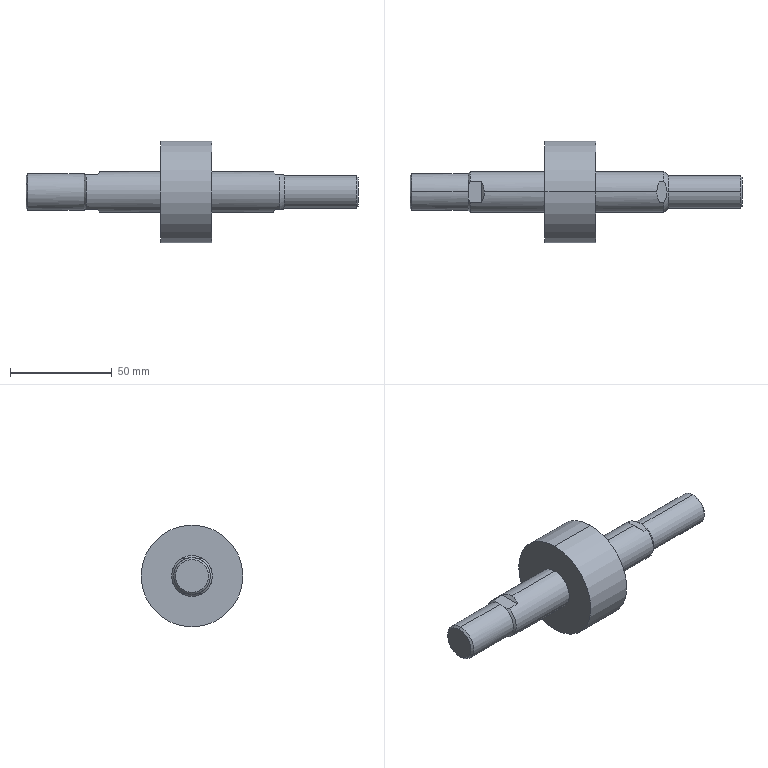Part | SolidWorks | features BaseBody 1 | 1 solid | 32 faces | box 163 x 50 x 50 mm | volume 86233 mm3 | plane 14 | cylinder 10 | cone 8 | commonest cylinder face diameters 20 x4 16 x2 18 x2 50 x2
STEP:
#1=CARTESIAN_POINT('',(57.75,0.,25.));
#2=VERTEX_POINT('',#1);
#3=CARTESIAN_POINT('',(57.75,0.,-25.));
#4=VERTEX_POINT('',#3);
#5=CARTESIAN_POINT('',(57.75,0.,0.));
#6=DIRECTION('',(-1.,0.,0.));
#7=DIRECTION('',(0.,0.,1.));
#8=AXIS2_PLACEMENT_3D('',#5,#6,#7);
#9=CIRCLE('',#8,25.);
#10=EDGE_CURVE('',#2,#4,#9,.T.);
#11=ORIENTED_EDGE('',*,*,#10,.T.);
#12=CARTESIAN_POINT('',(32.75,0.,-25.));
#13=VERTEX_POINT('',#12);
#14=CARTESIAN_POINT('',(57.75,0.,-25.));
#15=DIRECTION('',(-1.,0.,0.));
#16=VECTOR('',#15,1000.);
#17=LINE('',#14,#16);
#18=EDGE_CURVE('',#4,#13,#17,.T.);
#19=ORIENTED_EDGE('',*,*,#18,.T.);
#20=CARTESIAN_POINT('',(32.75,0.,25.));
#21=VERTEX_POINT('',#20);
#22=CARTESIAN_POINT('',(32.75,0.,0.));
#23=DIRECTION('',(1.,0.,0.));
#24=DIRECTION('',(0.,0.,1.));
#25=AXIS2_PLACEMENT_3D('',#22,#23,#24);
#26=CIRCLE('',#25,25.);
#27=EDGE_CURVE('',#13,#21,#26,.T.);
#28=ORIENTED_EDGE('',*,*,#27,.T.);
#29=CARTESIAN_POINT('',(57.75,0.,25.));
#30=DIRECTION('',(-1.,0.,0.));
#31=VECTOR('',#30,1000.);
#32=LINE('',#29,#31);
#33=EDGE_CURVE('',#2,#21,#32,.T.);
#34=ORIENTED_EDGE('',*,*,#33,.F.);
#35=EDGE_LOOP('',(#11,#19,#28,#34));
#36=FACE_OUTER_BOUND('',#35,.T.);
#37=CARTESIAN_POINT('',(57.75,0.,0.));
#38=DIRECTION('',(-1.,0.,0.));
#39=DIRECTION('',(0.,0.,1.));
#40=AXIS2_PLACEMENT_3D('',#37,#38,#39);
#41=CYLINDRICAL_SURFACE('',#40,25.);
#42=ADVANCED_FACE('',(#36),#41,.T.);
#43=CARTESIAN_POINT('',(32.75,0.,10.));
#44=VERTEX_POINT('',#43);
#45=CARTESIAN_POINT('',(32.75,0.,-10.));
#46=VERTEX_POINT('',#45);
#47=CARTESIAN_POINT('',(32.75,0.,0.));
#48=DIRECTION('',(-1.,0.,0.));
#49=DIRECTION('',(0.,0.,1.));
#50=AXIS2_PLACEMENT_3D('',#47,#48,#49);
#51=CIRCLE('',#50,10.);
#52=EDGE_CURVE('',#44,#46,#51,.T.);
#53=ORIENTED_EDGE('',*,*,#52,.T.);
#54=CARTESIAN_POINT('',(3.,0.,-10.));
#55=VERTEX_POINT('',#54);
#56=CARTESIAN_POINT('',(57.75,0.,-10.));
#57=DIRECTION('',(-1.,0.,0.));
#58=VECTOR('',#57,1000.);
#59=LINE('',#56,#58);
#60=EDGE_CURVE('',#46,#55,#59,.T.);
#61=ORIENTED_EDGE('',*,*,#60,.T.);
#62=CARTESIAN_POINT('',(1.5,5.268,-8.5));
#63=VERTEX_POINT('',#62);
#64=CARTESIAN_POINT('',(3.,0.,-10.));
#65=CARTESIAN_POINT('',(3.,1.873,-10.));
#66=CARTESIAN_POINT('',(2.487,3.675,-9.487));
#67=CARTESIAN_POINT('',(1.5,5.268,-8.5));
#68=(BOUNDED_CURVE()B_SPLINE_CURVE(3,(#64,#65,#66,#67),.UNSPECIFIED.,.F.,.F.)B_SPLINE_CURVE_WITH_KNOTS((4,4),(3.142,3.696),.UNSPECIFIED.)CURVE()GEOMETRIC_REPRESENTATION_ITEM()RATIONAL_B_SPLINE_CURVE((1.,0.9745,0.9745,1.))REPRESENTATION_ITEM(''));
#69=EDGE_CURVE('',#55,#63,#68,.T.);
#70=ORIENTED_EDGE('',*,*,#69,.T.);
#71=CARTESIAN_POINT('',(-4.,5.268,-8.5));
#72=VERTEX_POINT('',#71);
#73=CARTESIAN_POINT('',(57.75,5.268,-8.5));
#74=DIRECTION('',(-1.,0.,0.));
#75=VECTOR('',#74,1000.);
#76=LINE('',#73,#75);
#77=EDGE_CURVE('',#63,#72,#76,.T.);
#78=ORIENTED_EDGE('',*,*,#77,.T.);
#79=CARTESIAN_POINT('',(-4.,5.268,8.5));
#80=VERTEX_POINT('',#79);
#81=CARTESIAN_POINT('',(-4.,0.,0.));
#82=DIRECTION('',(1.,0.,0.));
#83=DIRECTION('',(0.,0.,1.));
#84=AXIS2_PLACEMENT_3D('',#81,#82,#83);
#85=CIRCLE('',#84,10.);
#86=EDGE_CURVE('',#72,#80,#85,.T.);
#87=ORIENTED_EDGE('',*,*,#86,.T.);
#88=CARTESIAN_POINT('',(1.5,5.268,8.5));
#89=VERTEX_POINT('',#88);
#90=CARTESIAN_POINT('',(57.75,5.268,8.5));
#91=DIRECTION('',(1.,0.,0.));
#92=VECTOR('',#91,1000.);
#93=LINE('',#90,#92);
#94=EDGE_CURVE('',#80,#89,#93,.T.);
#95=ORIENTED_EDGE('',*,*,#94,.T.);
#96=CARTESIAN_POINT('',(3.,0.,10.));
#97=VERTEX_POINT('',#96);
#98=CARTESIAN_POINT('',(1.5,5.268,8.5));
#99=CARTESIAN_POINT('',(2.487,3.675,9.487));
#100=CARTESIAN_POINT('',(3.,1.873,10.));
#101=CARTESIAN_POINT('',(3.,0.,10.));
#102=(BOUNDED_CURVE()B_SPLINE_CURVE(3,(#98,#99,#100,#101),.UNSPECIFIED.,.F.,.F.)B_SPLINE_CURVE_WITH_KNOTS((4,4),(2.587,3.142),.UNSPECIFIED.)CURVE()GEOMETRIC_REPRESENTATION_ITEM()RATIONAL_B_SPLINE_CURVE((1.,0.9745,0.9745,1.))REPRESENTATION_ITEM(''));
#103=EDGE_CURVE('',#89,#97,#102,.T.);
#104=ORIENTED_EDGE('',*,*,#103,.T.);
#105=CARTESIAN_POINT('',(57.75,0.,10.));
#106=DIRECTION('',(-1.,0.,0.));
#107=VECTOR('',#106,1000.);
#108=LINE('',#105,#107);
#109=EDGE_CURVE('',#44,#97,#108,.T.);
#110=ORIENTED_EDGE('',*,*,#109,.F.);
#111=EDGE_LOOP('',(#53,#61,#70,#78,#87,#95,#104,#110));
#112=FACE_OUTER_BOUND('',#111,.T.);
#113=CARTESIAN_POINT('',(57.75,0.,0.));
#114=DIRECTION('',(-1.,0.,0.));
#115=DIRECTION('',(0.,0.,1.));
#116=AXIS2_PLACEMENT_3D('',#113,#114,#115);
#117=CYLINDRICAL_SURFACE('',#116,10.);
#118=ADVANCED_FACE('',(#112),#117,.T.);
#119=CARTESIAN_POINT('',(89.2,5.268,-8.5));
#120=VERTEX_POINT('',#119);
#121=CARTESIAN_POINT('',(87.7,0.,-10.));
#122=VERTEX_POINT('',#121);
#123=CARTESIAN_POINT('',(89.2,5.268,-8.5));
#124=CARTESIAN_POINT('',(88.213,3.675,-9.487));
#125=CARTESIAN_POINT('',(87.7,1.873,-10.));
#126=CARTESIAN_POINT('',(87.7,0.,-10.));
#127=(BOUNDED_CURVE()B_SPLINE_CURVE(3,(#123,#124,#125,#126),.UNSPECIFIED.,.F.,.F.)B_SPLINE_CURVE_WITH_KNOTS((4,4),(5.728,6.283),.UNSPECIFIED.)CURVE()GEOMETRIC_REPRESENTATION_ITEM()RATIONAL_B_SPLINE_CURVE((1.,0.9745,0.9745,1.))REPRESENTATION_ITEM(''));
#128=EDGE_CURVE('',#120,#122,#127,.T.);
#129=ORIENTED_EDGE('',*,*,#128,.T.);
#130=CARTESIAN_POINT('',(57.75,0.,-10.));
#131=VERTEX_POINT('',#130);
#132=CARTESIAN_POINT('',(129.5,0.,-10.));
#133=DIRECTION('',(-1.,0.,0.));
#134=VECTOR('',#133,1000.);
#135=LINE('',#132,#134);
#136=EDGE_CURVE('',#122,#131,#135,.T.);
#137=ORIENTED_EDGE('',*,*,#136,.T.);
#138=CARTESIAN_POINT('',(57.75,0.,10.));
#139=VERTEX_POINT('',#138);
#140=CARTESIAN_POINT('',(57.75,0.,0.));
#141=DIRECTION('',(1.,0.,0.));
#142=DIRECTION('',(0.,0.,1.));
#143=AXIS2_PLACEMENT_3D('',#140,#141,#142);
#144=CIRCLE('',#143,10.);
#145=EDGE_CURVE('',#131,#139,#144,.T.);
#146=ORIENTED_EDGE('',*,*,#145,.T.);
#147=CARTESIAN_POINT('',(87.7,0.,10.));
#148=VERTEX_POINT('',#147);
#149=CARTESIAN_POINT('',(129.5,0.,10.));
#150=DIRECTION('',(-1.,0.,0.));
#151=VECTOR('',#150,1000.);
#152=LINE('',#149,#151);
#153=EDGE_CURVE('',#148,#139,#152,.T.);
#154=ORIENTED_EDGE('',*,*,#153,.F.);
#155=CARTESIAN_POINT('',(89.2,5.268,8.5));
#156=VERTEX_POINT('',#155);
#157=CARTESIAN_POINT('',(87.7,0.,10.));
#158=CARTESIAN_POINT('',(87.7,1.873,10.));
#159=CARTESIAN_POINT('',(88.213,3.675,9.487));
#160=CARTESIAN_POINT('',(89.2,5.268,8.5));
#161=(BOUNDED_CURVE()B_SPLINE_CURVE(3,(#157,#158,#159,#160),.UNSPECIFIED.,.F.,.F.)B_SPLINE_CURVE_WITH_KNOTS((4,4),(0.,0.5548),.UNSPECIFIED.)CURVE()GEOMETRIC_REPRESENTATION_ITEM()RATIONAL_B_SPLINE_CURVE((1.,0.9745,0.9745,1.))REPRESENTATION_ITEM(''));
#162=EDGE_CURVE('',#148,#156,#161,.T.);
#163=ORIENTED_EDGE('',*,*,#162,.T.);
#164=CARTESIAN_POINT('',(91.2,5.268,8.5));
#165=VERTEX_POINT('',#164);
#166=CARTESIAN_POINT('',(129.5,5.268,8.5));
#167=DIRECTION('',(1.,0.,0.));
#168=VECTOR('',#167,1000.);
#169=LINE('',#166,#168);
#170=EDGE_CURVE('',#156,#165,#169,.T.);
#171=ORIENTED_EDGE('',*,*,#170,.T.);
#172=CARTESIAN_POINT('',(91.2,5.268,-8.5));
#173=VERTEX_POINT('',#172);
#174=CARTESIAN_POINT('',(91.2,0.,0.));
#175=DIRECTION('',(-1.,0.,0.));
#176=DIRECTION('',(0.,0.,1.));
#177=AXIS2_PLACEMENT_3D('',#174,#175,#176);
#178=CIRCLE('',#177,10.);
#179=EDGE_CURVE('',#165,#173,#178,.T.);
#180=ORIENTED_EDGE('',*,*,#179,.T.);
#181=CARTESIAN_POINT('',(129.5,5.268,-8.5));
#182=DIRECTION('',(-1.,0.,0.));
#183=VECTOR('',#182,1000.);
#184=LINE('',#181,#183);
#185=EDGE_CURVE('',#173,#120,#184,.T.);
#186=ORIENTED_EDGE('',*,*,#185,.T.);
#187=EDGE_LOOP('',(#129,#137,#146,#154,#163,#171,#180,#186));
#188=FACE_OUTER_BOUND('',#187,.T.);
#189=CARTESIAN_POINT('',(129.5,0.,0.));
#190=DIRECTION('',(-1.,0.,0.));
#191=DIRECTION('',(0.,0.,1.));
#192=AXIS2_PLACEMENT_3D('',#189,#190,#191);
#193=CYLINDRICAL_SURFACE('',#192,10.);
#194=ADVANCED_FACE('',(#188),#193,.T.);
#195=CARTESIAN_POINT('',(93.2,0.,8.));
#196=VERTEX_POINT('',#195);
#197=CARTESIAN_POINT('',(93.2,0.,-8.));
#198=VERTEX_POINT('',#197);
#199=CARTESIAN_POINT('',(93.2,0.,0.));
#200=DIRECTION('',(-1.,0.,0.));
#201=DIRECTION('',(0.,0.,1.));
#202=AXIS2_PLACEMENT_3D('',#199,#200,#201);
#203=CIRCLE('',#202,8.);
#204=EDGE_CURVE('',#196,#198,#203,.T.);
#205=ORIENTED_EDGE('',*,*,#204,.T.);
#206=CARTESIAN_POINT('',(92.7,0.,-8.5));
#207=VERTEX_POINT('',#206);
#208=CARTESIAN_POINT('',(91.2,0.,-10.));
#209=DIRECTION('',(-0.7071,0.,-0.7071));
#210=VECTOR('',#209,1000.);
#211=LINE('',#208,#210);
#212=EDGE_CURVE('',#198,#207,#211,.T.);
#213=ORIENTED_EDGE('',*,*,#212,.T.);
#214=CARTESIAN_POINT('',(92.7,0.,-8.5));
#215=CARTESIAN_POINT('',(92.7,0.459,-8.5));
#216=CARTESIAN_POINT('',(92.663,0.9179,-8.5));
#217=CARTESIAN_POINT('',(92.516,1.835,-8.5));
#218=CARTESIAN_POINT('',(92.408,2.287,-8.5));
#219=CARTESIAN_POINT('',(92.005,3.607,-8.5));
#220=CARTESIAN_POINT('',(91.632,4.448,-8.5));
#221=CARTESIAN_POINT('',(91.2,5.268,-8.5));
#222=B_SPLINE_CURVE_WITH_KNOTS('',3,(#214,#215,#216,#217,#218,#219,#220,#221),.UNSPECIFIED.,.F.,.F.,(4,2,2,4),(0.005508,0.006884,0.008261,0.01101),.UNSPECIFIED.);
#223=EDGE_CURVE('',#207,#173,#222,.T.);
#224=ORIENTED_EDGE('',*,*,#223,.T.);
#225=ORIENTED_EDGE('',*,*,#179,.F.);
#226=CARTESIAN_POINT('',(92.7,0.,8.5));
#227=VERTEX_POINT('',#226);
#228=CARTESIAN_POINT('',(92.7,0.,8.5));
#229=CARTESIAN_POINT('',(92.7,0.459,8.5));
#230=CARTESIAN_POINT('',(92.663,0.9179,8.5));
#231=CARTESIAN_POINT('',(92.516,1.835,8.5));
#232=CARTESIAN_POINT('',(92.408,2.287,8.5));
#233=CARTESIAN_POINT('',(92.005,3.607,8.5));
#234=CARTESIAN_POINT('',(91.632,4.448,8.5));
#235=CARTESIAN_POINT('',(91.2,5.268,8.5));
#236=B_SPLINE_CURVE_WITH_KNOTS('',3,(#228,#229,#230,#231,#232,#233,#234,#235),.UNSPECIFIED.,.F.,.F.,(4,2,2,4),(0.005508,0.006884,0.008261,0.01101),.UNSPECIFIED.);
#237=EDGE_CURVE('',#227,#165,#236,.T.);
#238=ORIENTED_EDGE('',*,*,#237,.F.);
#239=CARTESIAN_POINT('',(91.2,0.,10.));
#240=DIRECTION('',(-0.7071,0.,0.7071));
#241=VECTOR('',#240,1000.);
#242=LINE('',#239,#241);
#243=EDGE_CURVE('',#196,#227,#242,.T.);
#244=ORIENTED_EDGE('',*,*,#243,.F.);
#245=EDGE_LOOP('',(#205,#213,#224,#225,#238,#244));
#246=FACE_OUTER_BOUND('',#245,.T.);
#247=CARTESIAN_POINT('',(91.2,0.,0.));
#248=DIRECTION('',(-1.,0.,0.));
#249=DIRECTION('',(0.,0.,1.));
#250=AXIS2_PLACEMENT_3D('',#247,#248,#249);
#251=CONICAL_SURFACE('',#250,10.,0.7854);
#252=ADVANCED_FACE('',(#246),#251,.T.);
#253=CARTESIAN_POINT('',(-5.,2.958,-8.5));
#254=VERTEX_POINT('',#253);
#255=CARTESIAN_POINT('',(-5.,0.,-9.));
#256=VERTEX_POINT('',#255);
#257=CARTESIAN_POINT('',(-5.,0.,0.));
#258=DIRECTION('',(-1.,0.,0.));
#259=DIRECTION('',(0.,0.,1.));
#260=AXIS2_PLACEMENT_3D('',#257,#258,#259);
#261=CIRCLE('',#260,9.);
#262=EDGE_CURVE('',#254,#256,#261,.T.);
#263=ORIENTED_EDGE('',*,*,#262,.T.);
#264=CARTESIAN_POINT('',(-32.58,0.,-9.));
#265=VERTEX_POINT('',#264);
#266=CARTESIAN_POINT('',(0.,0.,-9.));
#267=DIRECTION('',(-1.,0.,0.));
#268=VECTOR('',#267,1000.);
#269=LINE('',#266,#268);
#270=EDGE_CURVE('',#256,#265,#269,.T.);
#271=ORIENTED_EDGE('',*,*,#270,.T.);
#272=CARTESIAN_POINT('',(-32.58,0.,9.));
#273=VERTEX_POINT('',#272);
#274=CARTESIAN_POINT('',(-32.58,0.,0.));
#275=DIRECTION('',(1.,0.,0.));
#276=DIRECTION('',(0.,0.,1.));
#277=AXIS2_PLACEMENT_3D('',#274,#275,#276);
#278=CIRCLE('',#277,9.);
#279=EDGE_CURVE('',#265,#273,#278,.T.);
#280=ORIENTED_EDGE('',*,*,#279,.T.);
#281=CARTESIAN_POINT('',(-5.,0.,9.));
#282=VERTEX_POINT('',#281);
#283=CARTESIAN_POINT('',(0.,0.,9.));
#284=DIRECTION('',(-1.,0.,0.));
#285=VECTOR('',#284,1000.);
#286=LINE('',#283,#285);
#287=EDGE_CURVE('',#282,#273,#286,.T.);
#288=ORIENTED_EDGE('',*,*,#287,.F.);
#289=CARTESIAN_POINT('',(-5.,2.958,8.5));
#290=VERTEX_POINT('',#289);
#291=CARTESIAN_POINT('',(-5.,0.,0.));
#292=DIRECTION('',(1.,0.,0.));
#293=DIRECTION('',(0.,0.,1.));
#294=AXIS2_PLACEMENT_3D('',#291,#292,#293);
#295=CIRCLE('',#294,9.);
#296=EDGE_CURVE('',#290,#282,#295,.T.);
#297=ORIENTED_EDGE('',*,*,#296,.F.);
#298=CARTESIAN_POINT('',(-5.,0.,0.));
#299=DIRECTION('',(1.,0.,0.));
#300=DIRECTION('',(0.,0.,-1.));
#301=AXIS2_PLACEMENT_3D('',#298,#299,#300);
#302=CIRCLE('',#301,9.);
#303=EDGE_CURVE('',#254,#290,#302,.T.);
#304=ORIENTED_EDGE('',*,*,#303,.F.);
#305=EDGE_LOOP('',(#263,#271,#280,#288,#297,#304));
#306=FACE_OUTER_BOUND('',#305,.T.);
#307=CARTESIAN_POINT('',(0.,0.,0.));
#308=DIRECTION('',(-1.,0.,0.));
#309=DIRECTION('',(0.,0.,1.));
#310=AXIS2_PLACEMENT_3D('',#307,#308,#309);
#311=CYLINDRICAL_SURFACE('',#310,9.);
#312=ADVANCED_FACE('',(#306),#311,.T.);
#313=CARTESIAN_POINT('',(128.58,0.,8.));
#314=VERTEX_POINT('',#313);
#315=CARTESIAN_POINT('',(128.58,0.,-8.));
#316=VERTEX_POINT('',#315);
#317=CARTESIAN_POINT('',(128.58,0.,0.));
#318=DIRECTION('',(-1.,0.,0.));
#319=DIRECTION('',(0.,0.,1.));
#320=AXIS2_PLACEMENT_3D('',#317,#318,#319);
#321=CIRCLE('',#320,8.);
#322=EDGE_CURVE('',#314,#316,#321,.T.);
#323=ORIENTED_EDGE('',*,*,#322,.T.);
#324=CARTESIAN_POINT('',(129.5,0.,-8.));
#325=DIRECTION('',(-1.,0.,0.));
#326=VECTOR('',#325,1000.);
#327=LINE('',#324,#326);
#328=EDGE_CURVE('',#316,#198,#327,.T.);
#329=ORIENTED_EDGE('',*,*,#328,.T.);
#330=ORIENTED_EDGE('',*,*,#204,.F.);
#331=CARTESIAN_POINT('',(129.5,0.,8.));
#332=DIRECTION('',(-1.,0.,0.));
#333=VECTOR('',#332,1000.);
#334=LINE('',#331,#333);
#335=EDGE_CURVE('',#314,#196,#334,.T.);
#336=ORIENTED_EDGE('',*,*,#335,.F.);
#337=EDGE_LOOP('',(#323,#329,#330,#336));
#338=FACE_OUTER_BOUND('',#337,.T.);
#339=CARTESIAN_POINT('',(129.5,0.,0.));
#340=DIRECTION('',(-1.,0.,0.));
#341=DIRECTION('',(0.,0.,1.));
#342=AXIS2_PLACEMENT_3D('',#339,#340,#341);
#343=CYLINDRICAL_SURFACE('',#342,8.);
#344=ADVANCED_FACE('',(#338),#343,.T.);
#345=CARTESIAN_POINT('',(-33.5,0.,-8.08));
#346=VERTEX_POINT('',#345);
#347=CARTESIAN_POINT('',(-33.5,0.,8.08));
#348=VERTEX_POINT('',#347);
#349=CARTESIAN_POINT('',(-33.5,0.,0.));
#350=DIRECTION('',(1.,0.,0.));
#351=DIRECTION('',(0.,0.,-1.));
#352=AXIS2_PLACEMENT_3D('',#349,#350,#351);
#353=CIRCLE('',#352,8.08);
#354=EDGE_CURVE('',#346,#348,#353,.T.);
#355=ORIENTED_EDGE('',*,*,#354,.T.);
#356=CARTESIAN_POINT('',(-32.58,0.,9.));
#357=DIRECTION('',(0.7071,0.,0.7071));
#358=VECTOR('',#357,1000.);
#359=LINE('',#356,#358);
#360=EDGE_CURVE('',#348,#273,#359,.T.);
#361=ORIENTED_EDGE('',*,*,#360,.T.);
#362=ORIENTED_EDGE('',*,*,#279,.F.);
#363=CARTESIAN_POINT('',(-32.58,0.,-9.));
#364=DIRECTION('',(0.7071,0.,-0.7071));
#365=VECTOR('',#364,1000.);
#366=LINE('',#363,#365);
#367=EDGE_CURVE('',#346,#265,#366,.T.);
#368=ORIENTED_EDGE('',*,*,#367,.F.);
#369=EDGE_LOOP('',(#355,#361,#362,#368));
#370=FACE_OUTER_BOUND('',#369,.T.);
#371=CARTESIAN_POINT('',(-32.58,0.,0.));
#372=DIRECTION('',(1.,0.,0.));
#373=DIRECTION('',(0.,0.,-1.));
#374=AXIS2_PLACEMENT_3D('',#371,#372,#373);
#375=CONICAL_SURFACE('',#374,9.,0.7854);
#376=ADVANCED_FACE('',(#370),#375,.T.);
#377=CARTESIAN_POINT('',(129.5,0.,7.08));
#378=VERTEX_POINT('',#377);
#379=CARTESIAN_POINT('',(129.5,0.,-7.08));
#380=VERTEX_POINT('',#379);
#381=CARTESIAN_POINT('',(129.5,0.,0.));
#382=DIRECTION('',(-1.,0.,0.));
#383=DIRECTION('',(0.,0.,1.));
#384=AXIS2_PLACEMENT_3D('',#381,#382,#383);
#385=CIRCLE('',#384,7.08);
#386=EDGE_CURVE('',#378,#380,#385,.T.);
#387=ORIENTED_EDGE('',*,*,#386,.T.);
#388=CARTESIAN_POINT('',(128.58,0.,-8.));
#389=DIRECTION('',(-0.7071,0.,-0.7071));
#390=VECTOR('',#389,1000.);
#391=LINE('',#388,#390);
#392=EDGE_CURVE('',#380,#316,#391,.T.);
#393=ORIENTED_EDGE('',*,*,#392,.T.);
#394=ORIENTED_EDGE('',*,*,#322,.F.);
#395=CARTESIAN_POINT('',(128.58,0.,8.));
#396=DIRECTION('',(-0.7071,0.,0.7071));
#397=VECTOR('',#396,1000.);
#398=LINE('',#395,#397);
#399=EDGE_CURVE('',#378,#314,#398,.T.);
#400=ORIENTED_EDGE('',*,*,#399,.F.);
#401=EDGE_LOOP('',(#387,#393,#394,#400));
#402=FACE_OUTER_BOUND('',#401,.T.);
#403=CARTESIAN_POINT('',(128.58,0.,0.));
#404=DIRECTION('',(-1.,0.,0.));
#405=DIRECTION('',(0.,0.,1.));
#406=AXIS2_PLACEMENT_3D('',#403,#404,#405);
#407=CONICAL_SURFACE('',#406,8.,0.7854);
#408=ADVANCED_FACE('',(#402),#407,.T.);
#409=ORIENTED_EDGE('',*,*,#18,.F.);
#410=CARTESIAN_POINT('',(57.75,0.,0.));
#411=DIRECTION('',(-1.,0.,0.));
#412=DIRECTION('',(0.,0.,1.));
#413=AXIS2_PLACEMENT_3D('',#410,#411,#412);
#414=CIRCLE('',#413,25.);
#415=EDGE_CURVE('',#4,#2,#414,.T.);
#416=ORIENTED_EDGE('',*,*,#415,.T.);
#417=ORIENTED_EDGE('',*,*,#33,.T.);
#418=CARTESIAN_POINT('',(32.75,0.,0.));
#419=DIRECTION('',(1.,0.,0.));
#420=DIRECTION('',(0.,0.,1.));
#421=AXIS2_PLACEMENT_3D('',#418,#419,#420);
#422=CIRCLE('',#421,25.);
#423=EDGE_CURVE('',#21,#13,#422,.T.);
#424=ORIENTED_EDGE('',*,*,#423,.T.);
#425=EDGE_LOOP('',(#409,#416,#417,#424));
#426=FACE_OUTER_BOUND('',#425,.T.);
#427=CARTESIAN_POINT('',(57.75,0.,0.));
#428=DIRECTION('',(-1.,0.,0.));
#429=DIRECTION('',(0.,0.,1.));
#430=AXIS2_PLACEMENT_3D('',#427,#428,#429);
#431=CYLINDRICAL_SURFACE('',#430,25.);
#432=ADVANCED_FACE('',(#426),#431,.T.);
#433=ORIENTED_EDGE('',*,*,#52,.F.);
#434=CARTESIAN_POINT('',(32.75,0.,0.));
#435=DIRECTION('',(-1.,0.,0.));
#436=DIRECTION('',(0.,0.,1.));
#437=AXIS2_PLACEMENT_3D('',#434,#435,#436);
#438=CIRCLE('',#437,10.);
#439=EDGE_CURVE('',#46,#44,#438,.T.);
#440=ORIENTED_EDGE('',*,*,#439,.F.);
#441=EDGE_LOOP('',(#433,#440));
#442=FACE_BOUND('',#441,.T.);
#443=ORIENTED_EDGE('',*,*,#423,.F.);
#444=ORIENTED_EDGE('',*,*,#27,.F.);
#445=EDGE_LOOP('',(#443,#444));
#446=FACE_OUTER_BOUND('',#445,.T.);
#447=CARTESIAN_POINT('',(32.75,10.,0.));
#448=DIRECTION('',(1.,0.,0.));
#449=DIRECTION('',(0.,0.,-1.));
#450=AXIS2_PLACEMENT_3D('',#447,#448,#449);
#451=PLANE('',#450);
#452=ADVANCED_FACE('',(#442,#446),#451,.F.);
#453=ORIENTED_EDGE('',*,*,#10,.F.);
#454=ORIENTED_EDGE('',*,*,#415,.F.);
#455=EDGE_LOOP('',(#453,#454));
#456=FACE_OUTER_BOUND('',#455,.T.);
#457=CARTESIAN_POINT('',(57.75,0.,0.));
#458=DIRECTION('',(1.,0.,0.));
#459=DIRECTION('',(0.,0.,1.));
#460=AXIS2_PLACEMENT_3D('',#457,#458,#459);
#461=CIRCLE('',#460,10.);
#462=EDGE_CURVE('',#139,#131,#461,.T.);
#463=ORIENTED_EDGE('',*,*,#462,.F.);
#464=ORIENTED_EDGE('',*,*,#145,.F.);
#465=EDGE_LOOP('',(#463,#464));
#466=FACE_BOUND('',#465,.T.);
#467=CARTESIAN_POINT('',(57.75,25.,0.));
#468=DIRECTION('',(-1.,0.,0.));
#469=DIRECTION('',(0.,0.,1.));
#470=AXIS2_PLACEMENT_3D('',#467,#468,#469);
#471=PLANE('',#470);
#472=ADVANCED_FACE('',(#456,#466),#471,.F.);
#473=ORIENTED_EDGE('',*,*,#60,.F.);
#474=ORIENTED_EDGE('',*,*,#439,.T.);
#475=ORIENTED_EDGE('',*,*,#109,.T.);
#476=CARTESIAN_POINT('',(1.5,-5.268,8.5));
#477=VERTEX_POINT('',#476);
#478=CARTESIAN_POINT('',(3.,0.,10.));
#479=CARTESIAN_POINT('',(3.,-1.873,10.));
#480=CARTESIAN_POINT('',(2.487,-3.675,9.487));
#481=CARTESIAN_POINT('',(1.5,-5.268,8.5));
#482=(BOUNDED_CURVE()B_SPLINE_CURVE(3,(#478,#479,#480,#481),.UNSPECIFIED.,.F.,.F.)B_SPLINE_CURVE_WITH_KNOTS((4,4),(3.142,3.696),.UNSPECIFIED.)CURVE()GEOMETRIC_REPRESENTATION_ITEM()RATIONAL_B_SPLINE_CURVE((1.,0.9745,0.9745,1.))REPRESENTATION_ITEM(''));
#483=EDGE_CURVE('',#97,#477,#482,.T.);
#484=ORIENTED_EDGE('',*,*,#483,.T.);
#485=CARTESIAN_POINT('',(-4.,-5.268,8.5));
#486=VERTEX_POINT('',#485);
#487=CARTESIAN_POINT('',(57.75,-5.268,8.5));
#488=DIRECTION('',(-1.,0.,0.));
#489=VECTOR('',#488,1000.);
#490=LINE('',#487,#489);
#491=EDGE_CURVE('',#477,#486,#490,.T.);
#492=ORIENTED_EDGE('',*,*,#491,.T.);
#493=CARTESIAN_POINT('',(-4.,-5.268,-8.5));
#494=VERTEX_POINT('',#493);
#495=CARTESIAN_POINT('',(-4.,0.,0.));
#496=DIRECTION('',(1.,0.,0.));
#497=DIRECTION('',(0.,0.,1.));
#498=AXIS2_PLACEMENT_3D('',#495,#496,#497);
#499=CIRCLE('',#498,10.);
#500=EDGE_CURVE('',#486,#494,#499,.T.);
#501=ORIENTED_EDGE('',*,*,#500,.T.);
#502=CARTESIAN_POINT('',(1.5,-5.268,-8.5));
#503=VERTEX_POINT('',#502);
#504=CARTESIAN_POINT('',(57.75,-5.268,-8.5));
#505=DIRECTION('',(1.,0.,0.));
#506=VECTOR('',#505,1000.);
#507=LINE('',#504,#506);
#508=EDGE_CURVE('',#494,#503,#507,.T.);
#509=ORIENTED_EDGE('',*,*,#508,.T.);
#510=CARTESIAN_POINT('',(1.5,-5.268,-8.5));
#511=CARTESIAN_POINT('',(2.487,-3.675,-9.487));
#512=CARTESIAN_POINT('',(3.,-1.873,-10.));
#513=CARTESIAN_POINT('',(3.,0.,-10.));
#514=(BOUNDED_CURVE()B_SPLINE_CURVE(3,(#510,#511,#512,#513),.UNSPECIFIED.,.F.,.F.)B_SPLINE_CURVE_WITH_KNOTS((4,4),(2.587,3.142),.UNSPECIFIED.)CURVE()GEOMETRIC_REPRESENTATION_ITEM()RATIONAL_B_SPLINE_CURVE((1.,0.9745,0.9745,1.))REPRESENTATION_ITEM(''));
#515=EDGE_CURVE('',#503,#55,#514,.T.);
#516=ORIENTED_EDGE('',*,*,#515,.T.);
#517=EDGE_LOOP('',(#473,#474,#475,#484,#492,#501,#509,#516));
#518=FACE_OUTER_BOUND('',#517,.T.);
#519=CARTESIAN_POINT('',(57.75,0.,0.));
#520=DIRECTION('',(-1.,0.,0.));
#521=DIRECTION('',(0.,0.,1.));
#522=AXIS2_PLACEMENT_3D('',#519,#520,#521);
#523=CYLINDRICAL_SURFACE('',#522,10.);
#524=ADVANCED_FACE('',(#518),#523,.T.);
#525=ORIENTED_EDGE('',*,*,#136,.F.);
#526=CARTESIAN_POINT('',(89.2,-5.268,-8.5));
#527=VERTEX_POINT('',#526);
#528=CARTESIAN_POINT('',(87.7,0.,-10.));
#529=CARTESIAN_POINT('',(87.7,-1.873,-10.));
#530=CARTESIAN_POINT('',(88.213,-3.675,-9.487));
#531=CARTESIAN_POINT('',(89.2,-5.268,-8.5));
#532=(BOUNDED_CURVE()B_SPLINE_CURVE(3,(#528,#529,#530,#531),.UNSPECIFIED.,.F.,.F.)B_SPLINE_CURVE_WITH_KNOTS((4,4),(0.,0.5548),.UNSPECIFIED.)CURVE()GEOMETRIC_REPRESENTATION_ITEM()RATIONAL_B_SPLINE_CURVE((1.,0.9745,0.9745,1.))REPRESENTATION_ITEM(''));
#533=EDGE_CURVE('',#122,#527,#532,.T.);
#534=ORIENTED_EDGE('',*,*,#533,.T.);
#535=CARTESIAN_POINT('',(91.2,-5.268,-8.5));
#536=VERTEX_POINT('',#535);
#537=CARTESIAN_POINT('',(129.5,-5.268,-8.5));
#538=DIRECTION('',(1.,0.,0.));
#539=VECTOR('',#538,1000.);
#540=LINE('',#537,#539);
#541=EDGE_CURVE('',#527,#536,#540,.T.);
#542=ORIENTED_EDGE('',*,*,#541,.T.);
#543=CARTESIAN_POINT('',(91.2,-5.268,8.5));
#544=VERTEX_POINT('',#543);
#545=CARTESIAN_POINT('',(91.2,0.,0.));
#546=DIRECTION('',(-1.,0.,0.));
#547=DIRECTION('',(0.,0.,1.));
#548=AXIS2_PLACEMENT_3D('',#545,#546,#547);
#549=CIRCLE('',#548,10.);
#550=EDGE_CURVE('',#536,#544,#549,.T.);
#551=ORIENTED_EDGE('',*,*,#550,.T.);
#552=CARTESIAN_POINT('',(89.2,-5.268,8.5));
#553=VERTEX_POINT('',#552);
#554=CARTESIAN_POINT('',(129.5,-5.268,8.5));
#555=DIRECTION('',(-1.,0.,0.));
#556=VECTOR('',#555,1000.);
#557=LINE('',#554,#556);
#558=EDGE_CURVE('',#544,#553,#557,.T.);
#559=ORIENTED_EDGE('',*,*,#558,.T.);
#560=CARTESIAN_POINT('',(89.2,-5.268,8.5));
#561=CARTESIAN_POINT('',(88.213,-3.675,9.487));
#562=CARTESIAN_POINT('',(87.7,-1.873,10.));
#563=CARTESIAN_POINT('',(87.7,0.,10.));
#564=(BOUNDED_CURVE()B_SPLINE_CURVE(3,(#560,#561,#562,#563),.UNSPECIFIED.,.F.,.F.)B_SPLINE_CURVE_WITH_KNOTS((4,4),(5.728,6.283),.UNSPECIFIED.)CURVE()GEOMETRIC_REPRESENTATION_ITEM()RATIONAL_B_SPLINE_CURVE((1.,0.9745,0.9745,1.))REPRESENTATION_ITEM(''));
#565=EDGE_CURVE('',#553,#148,#564,.T.);
#566=ORIENTED_EDGE('',*,*,#565,.T.);
#567=ORIENTED_EDGE('',*,*,#153,.T.);
#568=ORIENTED_EDGE('',*,*,#462,.T.);
#569=EDGE_LOOP('',(#525,#534,#542,#551,#559,#566,#567,#568));
#570=FACE_OUTER_BOUND('',#569,.T.);
#571=CARTESIAN_POINT('',(129.5,0.,0.));
#572=DIRECTION('',(-1.,0.,0.));
#573=DIRECTION('',(0.,0.,1.));
#574=AXIS2_PLACEMENT_3D('',#571,#572,#573);
#575=CYLINDRICAL_SURFACE('',#574,10.);
#576=ADVANCED_FACE('',(#570),#575,.T.);
#577=ORIENTED_EDGE('',*,*,#103,.F.);
#578=CARTESIAN_POINT('',(1.5,17.,8.5));
#579=DIRECTION('',(0.,-1.,0.));
#580=VECTOR('',#579,1000.);
#581=LINE('',#578,#580);
#582=EDGE_CURVE('',#89,#477,#581,.T.);
#583=ORIENTED_EDGE('',*,*,#582,.T.);
#584=ORIENTED_EDGE('',*,*,#483,.F.);
#585=EDGE_LOOP('',(#577,#583,#584));
#586=FACE_OUTER_BOUND('',#585,.T.);
#587=CARTESIAN_POINT('',(21.5,17.,28.5));
#588=DIRECTION('',(-0.7071,0.,0.7071));
#589=DIRECTION('',(0.7071,0.,0.7071));
#590=AXIS2_PLACEMENT_3D('',#587,#588,#589);
#591=PLANE('',#590);
#592=ADVANCED_FACE('',(#586),#591,.T.);
#593=ORIENTED_EDGE('',*,*,#491,.F.);
#594=ORIENTED_EDGE('',*,*,#582,.F.);
#595=ORIENTED_EDGE('',*,*,#94,.F.);
#596=CARTESIAN_POINT('',(-4.,5.268,8.5));
#597=CARTESIAN_POINT('',(-4.392,4.523,8.5));
#598=CARTESIAN_POINT('',(-4.737,3.758,8.5));
#599=CARTESIAN_POINT('',(-5.,2.958,8.5));
#600=B_SPLINE_CURVE_WITH_KNOTS('',3,(#596,#597,#598,#599),.UNSPECIFIED.,.F.,.F.,(4,4),(0.,0.002517),.UNSPECIFIED.);
#601=EDGE_CURVE('',#80,#290,#600,.T.);
#602=ORIENTED_EDGE('',*,*,#601,.T.);
#603=CARTESIAN_POINT('',(-5.,-2.958,8.5));
#604=VERTEX_POINT('',#603);
#605=CARTESIAN_POINT('',(-5.,17.,8.5));
#606=DIRECTION('',(0.,-1.,0.));
#607=VECTOR('',#606,1000.);
#608=LINE('',#605,#607);
#609=EDGE_CURVE('',#290,#604,#608,.T.);
#610=ORIENTED_EDGE('',*,*,#609,.T.);
#611=CARTESIAN_POINT('',(-5.,-2.958,8.5));
#612=CARTESIAN_POINT('',(-4.737,-3.758,8.5));
#613=CARTESIAN_POINT('',(-4.392,-4.523,8.5));
#614=CARTESIAN_POINT('',(-4.,-5.268,8.5));
#615=B_SPLINE_CURVE_WITH_KNOTS('',3,(#611,#612,#613,#614),.UNSPECIFIED.,.F.,.F.,(4,4),(0.,0.002517),.UNSPECIFIED.);
#616=EDGE_CURVE('',#604,#486,#615,.T.);
#617=ORIENTED_EDGE('',*,*,#616,.T.);
#618=EDGE_LOOP('',(#593,#594,#595,#602,#610,#617));
#619=FACE_OUTER_BOUND('',#618,.T.);
#620=CARTESIAN_POINT('',(1.5,17.,8.5));
#621=DIRECTION('',(0.,0.,1.));
#622=DIRECTION('',(1.,0.,0.));
#623=AXIS2_PLACEMENT_3D('',#620,#621,#622);
#624=PLANE('',#623);
#625=ADVANCED_FACE('',(#619),#624,.T.);
#626=ORIENTED_EDGE('',*,*,#601,.F.);
#627=ORIENTED_EDGE('',*,*,#86,.F.);
#628=CARTESIAN_POINT('',(-4.,5.268,-8.5));
#629=CARTESIAN_POINT('',(-4.392,4.523,-8.5));
#630=CARTESIAN_POINT('',(-4.737,3.758,-8.5));
#631=CARTESIAN_POINT('',(-5.,2.958,-8.5));
#632=B_SPLINE_CURVE_WITH_KNOTS('',3,(#628,#629,#630,#631),.UNSPECIFIED.,.F.,.F.,(4,4),(0.,0.002517),.UNSPECIFIED.);
#633=EDGE_CURVE('',#72,#254,#632,.T.);
#634=ORIENTED_EDGE('',*,*,#633,.T.);
#635=ORIENTED_EDGE('',*,*,#303,.T.);
#636=EDGE_LOOP('',(#626,#627,#634,#635));
#637=FACE_OUTER_BOUND('',#636,.T.);
#638=CARTESIAN_POINT('',(-4.,0.,0.));
#639=DIRECTION('',(1.,0.,0.));
#640=DIRECTION('',(0.,0.,-1.));
#641=AXIS2_PLACEMENT_3D('',#638,#639,#640);
#642=CONICAL_SURFACE('',#641,10.,0.7854);
#643=ADVANCED_FACE('',(#637),#642,.T.);
#644=ORIENTED_EDGE('',*,*,#77,.F.);
#645=CARTESIAN_POINT('',(1.5,17.,-8.5));
#646=DIRECTION('',(0.,-1.,0.));
#647=VECTOR('',#646,1000.);
#648=LINE('',#645,#647);
#649=EDGE_CURVE('',#63,#503,#648,.T.);
#650=ORIENTED_EDGE('',*,*,#649,.T.);
#651=ORIENTED_EDGE('',*,*,#508,.F.);
#652=CARTESIAN_POINT('',(-5.,-2.958,-8.5));
#653=VERTEX_POINT('',#652);
#654=CARTESIAN_POINT('',(-4.,-5.268,-8.5));
#655=CARTESIAN_POINT('',(-4.392,-4.523,-8.5));
#656=CARTESIAN_POINT('',(-4.737,-3.758,-8.5));
#657=CARTESIAN_POINT('',(-5.,-2.958,-8.5));
#658=B_SPLINE_CURVE_WITH_KNOTS('',3,(#654,#655,#656,#657),.UNSPECIFIED.,.F.,.F.,(4,4),(0.,0.002517),.UNSPECIFIED.);
#659=EDGE_CURVE('',#494,#653,#658,.T.);
#660=ORIENTED_EDGE('',*,*,#659,.T.);
#661=CARTESIAN_POINT('',(-5.,17.,-8.5));
#662=DIRECTION('',(0.,1.,0.));
#663=VECTOR('',#662,1000.);
#664=LINE('',#661,#663);
#665=EDGE_CURVE('',#653,#254,#664,.T.);
#666=ORIENTED_EDGE('',*,*,#665,.T.);
#667=ORIENTED_EDGE('',*,*,#633,.F.);
#668=EDGE_LOOP('',(#644,#650,#651,#660,#666,#667));
#669=FACE_OUTER_BOUND('',#668,.T.);
#670=CARTESIAN_POINT('',(-5.,17.,-8.5));
#671=DIRECTION('',(0.,0.,-1.));
#672=DIRECTION('',(-1.,0.,0.));
#673=AXIS2_PLACEMENT_3D('',#670,#671,#672);
#674=PLANE('',#673);
#675=ADVANCED_FACE('',(#669),#674,.T.);
#676=ORIENTED_EDGE('',*,*,#515,.F.);
#677=ORIENTED_EDGE('',*,*,#649,.F.);
#678=ORIENTED_EDGE('',*,*,#69,.F.);
#679=EDGE_LOOP('',(#676,#677,#678));
#680=FACE_OUTER_BOUND('',#679,.T.);
#681=CARTESIAN_POINT('',(1.5,17.,-8.5));
#682=DIRECTION('',(-0.7071,0.,-0.7071));
#683=DIRECTION('',(-0.7071,0.,0.7071));
#684=AXIS2_PLACEMENT_3D('',#681,#682,#683);
#685=PLANE('',#684);
#686=ADVANCED_FACE('',(#680),#685,.T.);
#687=ORIENTED_EDGE('',*,*,#659,.F.);
#688=ORIENTED_EDGE('',*,*,#500,.F.);
#689=ORIENTED_EDGE('',*,*,#616,.F.);
#690=CARTESIAN_POINT('',(-5.,0.,0.));
#691=DIRECTION('',(1.,0.,0.));
#692=DIRECTION('',(0.,0.,-1.));
#693=AXIS2_PLACEMENT_3D('',#690,#691,#692);
#694=CIRCLE('',#693,9.);
#695=EDGE_CURVE('',#604,#653,#694,.T.);
#696=ORIENTED_EDGE('',*,*,#695,.T.);
#697=EDGE_LOOP('',(#687,#688,#689,#696));
#698=FACE_OUTER_BOUND('',#697,.T.);
#699=CARTESIAN_POINT('',(-4.,0.,0.));
#700=DIRECTION('',(1.,0.,0.));
#701=DIRECTION('',(0.,0.,-1.));
#702=AXIS2_PLACEMENT_3D('',#699,#700,#701);
#703=CONICAL_SURFACE('',#702,10.,0.7854);
#704=ADVANCED_FACE('',(#698),#703,.T.);
#705=ORIENTED_EDGE('',*,*,#170,.F.);
#706=CARTESIAN_POINT('',(89.2,17.,8.5));
#707=DIRECTION('',(0.,-1.,0.));
#708=VECTOR('',#707,1000.);
#709=LINE('',#706,#708);
#710=EDGE_CURVE('',#156,#553,#709,.T.);
#711=ORIENTED_EDGE('',*,*,#710,.T.);
#712=ORIENTED_EDGE('',*,*,#558,.F.);
#713=CARTESIAN_POINT('',(91.2,-5.268,8.5));
#714=CARTESIAN_POINT('',(91.632,-4.448,8.5));
#715=CARTESIAN_POINT('',(92.004,-3.607,8.5));
#716=CARTESIAN_POINT('',(92.407,-2.288,8.5));
#717=CARTESIAN_POINT('',(92.516,-1.837,8.5));
#718=CARTESIAN_POINT('',(92.663,-0.9184,8.5));
#719=CARTESIAN_POINT('',(92.7,-0.4592,8.5));
#720=CARTESIAN_POINT('',(92.7,0.,8.5));
#721=B_SPLINE_CURVE_WITH_KNOTS('',3,(#713,#714,#715,#716,#717,#718,#719,#720),.UNSPECIFIED.,.F.,.F.,(4,2,2,4),(0.,0.002754,0.004131,0.005508),.UNSPECIFIED.);
#722=EDGE_CURVE('',#544,#227,#721,.T.);
#723=ORIENTED_EDGE('',*,*,#722,.T.);
#724=ORIENTED_EDGE('',*,*,#237,.T.);
#725=EDGE_LOOP('',(#705,#711,#712,#723,#724));
#726=FACE_OUTER_BOUND('',#725,.T.);
#727=CARTESIAN_POINT('',(93.2,17.,8.5));
#728=DIRECTION('',(0.,0.,1.));
#729=DIRECTION('',(1.,0.,0.));
#730=AXIS2_PLACEMENT_3D('',#727,#728,#729);
#731=PLANE('',#730);
#732=ADVANCED_FACE('',(#726),#731,.T.);
#733=ORIENTED_EDGE('',*,*,#565,.F.);
#734=ORIENTED_EDGE('',*,*,#710,.F.);
#735=ORIENTED_EDGE('',*,*,#162,.F.);
#736=EDGE_LOOP('',(#733,#734,#735));
#737=FACE_OUTER_BOUND('',#736,.T.);
#738=CARTESIAN_POINT('',(89.2,17.,8.5));
#739=DIRECTION('',(0.7071,0.,0.7071));
#740=DIRECTION('',(0.7071,0.,-0.7071));
#741=AXIS2_PLACEMENT_3D('',#738,#739,#740);
#742=PLANE('',#741);
#743=ADVANCED_FACE('',(#737),#742,.T.);
#744=ORIENTED_EDGE('',*,*,#212,.F.);
#745=CARTESIAN_POINT('',(93.2,0.,0.));
#746=DIRECTION('',(-1.,0.,0.));
#747=DIRECTION('',(0.,0.,1.));
#748=AXIS2_PLACEMENT_3D('',#745,#746,#747);
#749=CIRCLE('',#748,8.);
#750=EDGE_CURVE('',#198,#196,#749,.T.);
#751=ORIENTED_EDGE('',*,*,#750,.T.);
#752=ORIENTED_EDGE('',*,*,#243,.T.);
#753=ORIENTED_EDGE('',*,*,#722,.F.);
#754=ORIENTED_EDGE('',*,*,#550,.F.);
#755=CARTESIAN_POINT('',(91.2,-5.268,-8.5));
#756=CARTESIAN_POINT('',(91.632,-4.448,-8.5));
#757=CARTESIAN_POINT('',(92.004,-3.607,-8.5));
#758=CARTESIAN_POINT('',(92.407,-2.288,-8.5));
#759=CARTESIAN_POINT('',(92.516,-1.837,-8.5));
#760=CARTESIAN_POINT('',(92.663,-0.9184,-8.5));
#761=CARTESIAN_POINT('',(92.7,-0.4592,-8.5));
#762=CARTESIAN_POINT('',(92.7,0.,-8.5));
#763=B_SPLINE_CURVE_WITH_KNOTS('',3,(#755,#756,#757,#758,#759,#760,#761,#762),.UNSPECIFIED.,.F.,.F.,(4,2,2,4),(0.,0.002754,0.004131,0.005508),.UNSPECIFIED.);
#764=EDGE_CURVE('',#536,#207,#763,.T.);
#765=ORIENTED_EDGE('',*,*,#764,.T.);
#766=EDGE_LOOP('',(#744,#751,#752,#753,#754,#765));
#767=FACE_OUTER_BOUND('',#766,.T.);
#768=CARTESIAN_POINT('',(91.2,0.,0.));
#769=DIRECTION('',(-1.,0.,0.));
#770=DIRECTION('',(0.,0.,1.));
#771=AXIS2_PLACEMENT_3D('',#768,#769,#770);
#772=CONICAL_SURFACE('',#771,10.,0.7854);
#773=ADVANCED_FACE('',(#767),#772,.T.);
#774=ORIENTED_EDGE('',*,*,#541,.F.);
#775=CARTESIAN_POINT('',(89.2,17.,-8.5));
#776=DIRECTION('',(0.,1.,0.));
#777=VECTOR('',#776,1000.);
#778=LINE('',#775,#777);
#779=EDGE_CURVE('',#527,#120,#778,.T.);
#780=ORIENTED_EDGE('',*,*,#779,.T.);
#781=ORIENTED_EDGE('',*,*,#185,.F.);
#782=ORIENTED_EDGE('',*,*,#223,.F.);
#783=ORIENTED_EDGE('',*,*,#764,.F.);
#784=EDGE_LOOP('',(#774,#780,#781,#782,#783));
#785=FACE_OUTER_BOUND('',#784,.T.);
#786=CARTESIAN_POINT('',(89.2,17.,-8.5));
#787=DIRECTION('',(0.,0.,-1.));
#788=DIRECTION('',(-1.,0.,0.));
#789=AXIS2_PLACEMENT_3D('',#786,#787,#788);
#790=PLANE('',#789);
#791=ADVANCED_FACE('',(#785),#790,.T.);
#792=ORIENTED_EDGE('',*,*,#128,.F.);
#793=ORIENTED_EDGE('',*,*,#779,.F.);
#794=ORIENTED_EDGE('',*,*,#533,.F.);
#795=EDGE_LOOP('',(#792,#793,#794));
#796=FACE_OUTER_BOUND('',#795,.T.);
#797=CARTESIAN_POINT('',(82.129,17.,-15.571));
#798=DIRECTION('',(0.7071,0.,-0.7071));
#799=DIRECTION('',(-0.7071,0.,-0.7071));
#800=AXIS2_PLACEMENT_3D('',#797,#798,#799);
#801=PLANE('',#800);
#802=ADVANCED_FACE('',(#796),#801,.T.);
#803=ORIENTED_EDGE('',*,*,#296,.T.);
#804=CARTESIAN_POINT('',(-5.,0.,0.));
#805=DIRECTION('',(1.,0.,0.));
#806=DIRECTION('',(0.,0.,1.));
#807=AXIS2_PLACEMENT_3D('',#804,#805,#806);
#808=CIRCLE('',#807,9.);
#809=EDGE_CURVE('',#282,#604,#808,.T.);
#810=ORIENTED_EDGE('',*,*,#809,.T.);
#811=ORIENTED_EDGE('',*,*,#609,.F.);
#812=EDGE_LOOP('',(#803,#810,#811));
#813=FACE_OUTER_BOUND('',#812,.T.);
#814=CARTESIAN_POINT('',(-5.,17.,8.5));
#815=DIRECTION('',(1.,0.,0.));
#816=DIRECTION('',(0.,0.,-1.));
#817=AXIS2_PLACEMENT_3D('',#814,#815,#816);
#818=PLANE('',#817);
#819=ADVANCED_FACE('',(#813),#818,.T.);
#820=ORIENTED_EDGE('',*,*,#270,.F.);
#821=CARTESIAN_POINT('',(-5.,0.,0.));
#822=DIRECTION('',(-1.,0.,0.));
#823=DIRECTION('',(0.,0.,1.));
#824=AXIS2_PLACEMENT_3D('',#821,#822,#823);
#825=CIRCLE('',#824,9.);
#826=EDGE_CURVE('',#256,#653,#825,.T.);
#827=ORIENTED_EDGE('',*,*,#826,.T.);
#828=ORIENTED_EDGE('',*,*,#695,.F.);
#829=ORIENTED_EDGE('',*,*,#809,.F.);
#830=ORIENTED_EDGE('',*,*,#287,.T.);
#831=CARTESIAN_POINT('',(-32.58,0.,0.));
#832=DIRECTION('',(1.,0.,0.));
#833=DIRECTION('',(0.,0.,1.));
#834=AXIS2_PLACEMENT_3D('',#831,#832,#833);
#835=CIRCLE('',#834,9.);
#836=EDGE_CURVE('',#273,#265,#835,.T.);
#837=ORIENTED_EDGE('',*,*,#836,.T.);
#838=EDGE_LOOP('',(#820,#827,#828,#829,#830,#837));
#839=FACE_OUTER_BOUND('',#838,.T.);
#840=CARTESIAN_POINT('',(0.,0.,0.));
#841=DIRECTION('',(-1.,0.,0.));
#842=DIRECTION('',(0.,0.,1.));
#843=AXIS2_PLACEMENT_3D('',#840,#841,#842);
#844=CYLINDRICAL_SURFACE('',#843,9.);
#845=ADVANCED_FACE('',(#839),#844,.T.);
#846=ORIENTED_EDGE('',*,*,#262,.F.);
#847=ORIENTED_EDGE('',*,*,#665,.F.);
#848=ORIENTED_EDGE('',*,*,#826,.F.);
#849=EDGE_LOOP('',(#846,#847,#848));
#850=FACE_OUTER_BOUND('',#849,.T.);
#851=CARTESIAN_POINT('',(-5.,17.,-18.5));
#852=DIRECTION('',(1.,0.,0.));
#853=DIRECTION('',(0.,0.,-1.));
#854=AXIS2_PLACEMENT_3D('',#851,#852,#853);
#855=PLANE('',#854);
#856=ADVANCED_FACE('',(#850),#855,.T.);
#857=ORIENTED_EDGE('',*,*,#328,.F.);
#858=CARTESIAN_POINT('',(128.58,0.,0.));
#859=DIRECTION('',(-1.,0.,0.));
#860=DIRECTION('',(0.,0.,1.));
#861=AXIS2_PLACEMENT_3D('',#858,#859,#860);
#862=CIRCLE('',#861,8.);
#863=EDGE_CURVE('',#316,#314,#862,.T.);
#864=ORIENTED_EDGE('',*,*,#863,.T.);
#865=ORIENTED_EDGE('',*,*,#335,.T.);
#866=ORIENTED_EDGE('',*,*,#750,.F.);
#867=EDGE_LOOP('',(#857,#864,#865,#866));
#868=FACE_OUTER_BOUND('',#867,.T.);
#869=CARTESIAN_POINT('',(129.5,0.,0.));
#870=DIRECTION('',(-1.,0.,0.));
#871=DIRECTION('',(0.,0.,1.));
#872=AXIS2_PLACEMENT_3D('',#869,#870,#871);
#873=CYLINDRICAL_SURFACE('',#872,8.);
#874=ADVANCED_FACE('',(#868),#873,.T.);
#875=ORIENTED_EDGE('',*,*,#360,.F.);
#876=CARTESIAN_POINT('',(-33.5,0.,0.));
#877=DIRECTION('',(1.,0.,0.));
#878=DIRECTION('',(0.,0.,-1.));
#879=AXIS2_PLACEMENT_3D('',#876,#877,#878);
#880=CIRCLE('',#879,8.08);
#881=EDGE_CURVE('',#348,#346,#880,.T.);
#882=ORIENTED_EDGE('',*,*,#881,.T.);
#883=ORIENTED_EDGE('',*,*,#367,.T.);
#884=ORIENTED_EDGE('',*,*,#836,.F.);
#885=EDGE_LOOP('',(#875,#882,#883,#884));
#886=FACE_OUTER_BOUND('',#885,.T.);
#887=CARTESIAN_POINT('',(-32.58,0.,0.));
#888=DIRECTION('',(1.,0.,0.));
#889=DIRECTION('',(0.,0.,-1.));
#890=AXIS2_PLACEMENT_3D('',#887,#888,#889);
#891=CONICAL_SURFACE('',#890,9.,0.7854);
#892=ADVANCED_FACE('',(#886),#891,.T.);
#893=ORIENTED_EDGE('',*,*,#392,.F.);
#894=CARTESIAN_POINT('',(129.5,0.,0.));
#895=DIRECTION('',(-1.,0.,0.));
#896=DIRECTION('',(0.,0.,1.));
#897=AXIS2_PLACEMENT_3D('',#894,#895,#896);
#898=CIRCLE('',#897,7.08);
#899=EDGE_CURVE('',#380,#378,#898,.T.);
#900=ORIENTED_EDGE('',*,*,#899,.T.);
#901=ORIENTED_EDGE('',*,*,#399,.T.);
#902=ORIENTED_EDGE('',*,*,#863,.F.);
#903=EDGE_LOOP('',(#893,#900,#901,#902));
#904=FACE_OUTER_BOUND('',#903,.T.);
#905=CARTESIAN_POINT('',(128.58,0.,0.));
#906=DIRECTION('',(-1.,0.,0.));
#907=DIRECTION('',(0.,0.,1.));
#908=AXIS2_PLACEMENT_3D('',#905,#906,#907);
#909=CONICAL_SURFACE('',#908,8.,0.7854);
#910=ADVANCED_FACE('',(#904),#909,.T.);
#911=ORIENTED_EDGE('',*,*,#354,.F.);
#912=ORIENTED_EDGE('',*,*,#881,.F.);
#913=EDGE_LOOP('',(#911,#912));
#914=FACE_OUTER_BOUND('',#913,.T.);
#915=CARTESIAN_POINT('',(-33.5,0.,0.));
#916=DIRECTION('',(1.,0.,0.));
#917=DIRECTION('',(0.,0.,-1.));
#918=AXIS2_PLACEMENT_3D('',#915,#916,#917);
#919=PLANE('',#918);
#920=ADVANCED_FACE('',(#914),#919,.F.);
#921=ORIENTED_EDGE('',*,*,#386,.F.);
#922=ORIENTED_EDGE('',*,*,#899,.F.);
#923=EDGE_LOOP('',(#921,#922));
#924=FACE_OUTER_BOUND('',#923,.T.);
#925=CARTESIAN_POINT('',(129.5,7.08,0.));
#926=DIRECTION('',(-1.,0.,0.));
#927=DIRECTION('',(0.,0.,1.));
#928=AXIS2_PLACEMENT_3D('',#925,#926,#927);
#929=PLANE('',#928);
#930=ADVANCED_FACE('',(#924),#929,.F.);
#931=CLOSED_SHELL('',(#42,#118,#194,#252,#312,#344,#376,#408,#432,#452,#472,#524,#576,#592,#625,#643,#675,#686,#704,#732,#743,#773,#791,#802,#819,#845,#856,#874,#892,#910,#920,#930));
#932=MANIFOLD_SOLID_BREP('',#931);
#933=CARTESIAN_POINT('',(0.,0.,0.));
#934=DIRECTION('',(0.,0.,1.));
#935=DIRECTION('',(1.,0.,0.));
#936=AXIS2_PLACEMENT_3D('',#933,#934,#935);
#937=(LENGTH_UNIT()NAMED_UNIT(*)SI_UNIT(.MILLI.,.METRE.));
#938=UNCERTAINTY_MEASURE_WITH_UNIT(LENGTH_MEASURE(0.00001),#937,'','');
#939=(NAMED_UNIT(*)PLANE_ANGLE_UNIT()SI_UNIT($,.RADIAN.));
#940=(NAMED_UNIT(*)SI_UNIT($,.STERADIAN.)SOLID_ANGLE_UNIT());
#941=(GEOMETRIC_REPRESENTATION_CONTEXT(3)GLOBAL_UNCERTAINTY_ASSIGNED_CONTEXT((#938))GLOBAL_UNIT_ASSIGNED_CONTEXT((#937,#939,#940))REPRESENTATION_CONTEXT('',''));
#942=ADVANCED_BREP_SHAPE_REPRESENTATION('',(#932,#936),#941);